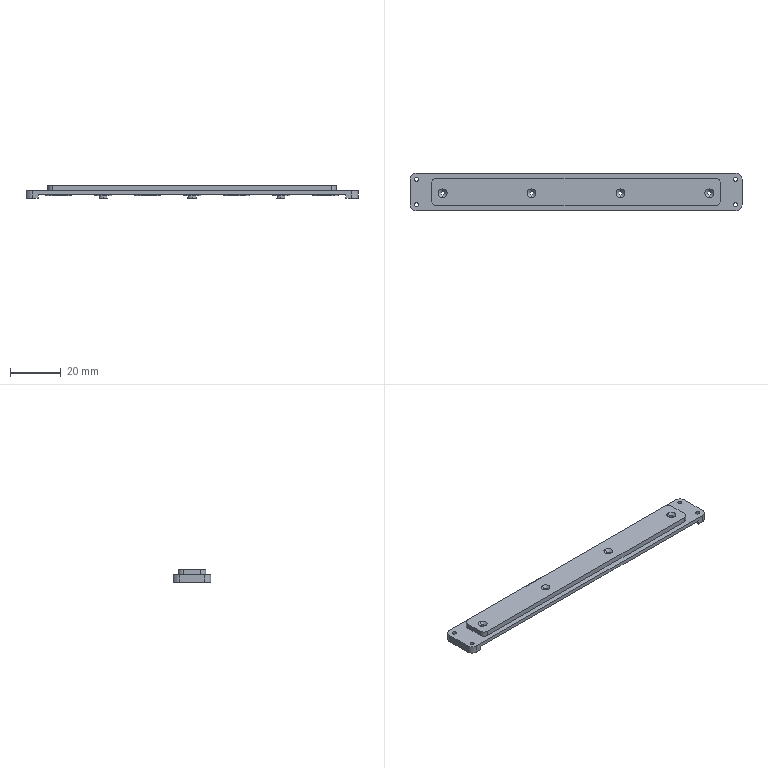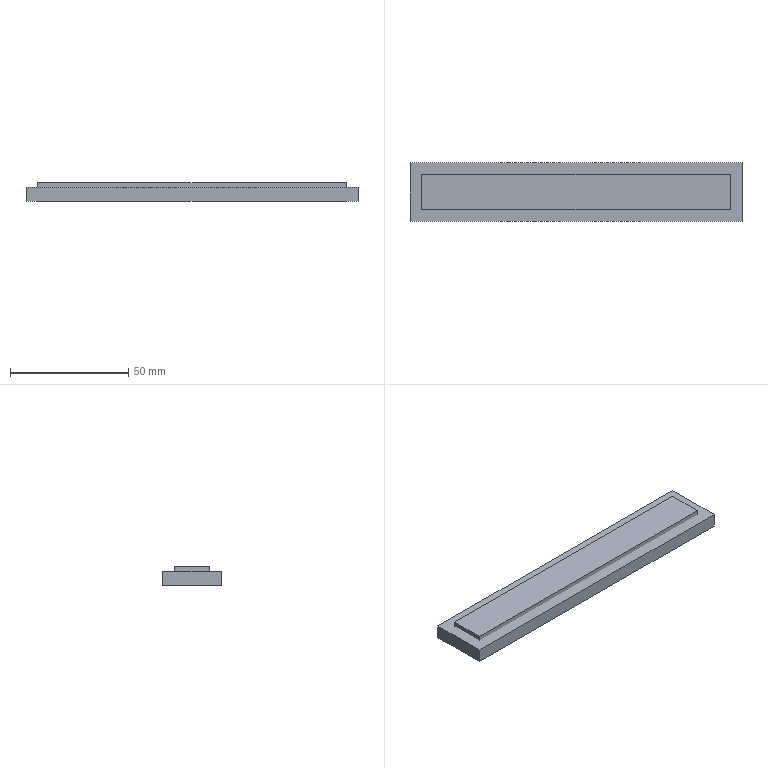CAM job | NX | 3-axis milling, drilling | part box 130.666 x 14.95 x 5 mm | stock box 140.666 x 24.95 x 8 mm
Tools:
number,name,description,diameter,corner_radius,flute_length,length,flutes
19,D80,Milling Tool-5 Parameters,80.0,0.0,50.0,75.0,2
1,D6A45,Milling Tool-5 Parameters,6.0,0.0,50.0,75.0,2
16,1.5ZT,Drilling Tool,1.5,0.0,35.0,50.0,2
17,1.6ZT,Drilling Tool,1.6,0.0,35.0,50.0,2
15,D10,Milling Tool-5 Parameters,10.0,0.0,50.0,75.0,2
14,D10JING,Milling Tool-5 Parameters,10.0,0.0,50.0,75.0,2
11,D4,Milling Tool-5 Parameters,4.0,0.0,50.0,75.0,2
2,D2,Milling Tool-5 Parameters,2.0,0.0,50.0,75.0,2
Operations:
program,operation,operation_type,tool,method,geometry_group,spindle_rpm,surface_speed,feed_per_tooth,feed_cut,feed_plunge,cut_length_mm,path_length_mm,cut_time_min,machine_time_min
1,FLOOR_WALL_COPY,VolumeBased25DMillingOperation,D80,METHOD,A,6500.0,1633.0,0.1154,1500.0,100.0,236.666,290.666,0.1578,0.1632
1,DRILLING_COPY_1,Operation,D6A45,METHOD,A,5000.0,94.0,0.035,350.0,0.0,38.0,306.457,0.1086,0.1354
1,DRILLING_COPY_1_COPY,Operation,1.5ZT,METHOD,A,2000.0,9.0,0.025,100.0,0.0,29.003,232.39,0.29,0.3104
1,DRILLING_COPY_1_COPY_COPY,Operation,1.6ZT,METHOD,A,2000.0,9.0,0.025,100.0,0.0,39.923,295.726,0.3992,0.4248
1,ADAPTIVE_MILLING,CavityMilling,D10,METHOD,A,9500.0,298.0,0.1579,3000.0,1000.0,3539.432,3666.063,1.184,1.196
1,ZLEVEL_PROFILE_COPY_1_COPY_COPY_1,ZLevelMilling,D10JING,METHOD,A,9500.0,298.0,0.0632,1200.0,1000.0,325.748,393.748,0.2721,0.2789
1,ZLEVEL_PROFILE_COPY_1_COPY_COPY_1_COPY,ZLevelMilling,D10JING,METHOD,A,9500.0,298.0,0.0632,1200.0,1000.0,284.366,346.366,0.2376,0.2438
1,PLANAR_MILL_COPY_COPY_COPY_COPY_COPY_COPY_1,PlanarMilling,D6A45,METHOD,A,9500.0,179.0,0.0658,1250.0,100.0,257.932,316.932,0.2063,0.2122
1,PLANAR_MILL_COPY_COPY_COPY_COPY_COPY_COPY_1_COPY,PlanarMilling,D6A45,METHOD,A,9500.0,179.0,0.0658,1250.0,100.0,308.731,374.731,0.247,0.2536
1,DRILLING_COPY_1_COPY_1,Operation,D6A45,METHOD,A,5000.0,94.0,0.035,350.0,0.0,16.4,252.287,0.0469,0.0704
2,FLOOR_WALL_COPY_COPY,VolumeBased25DMillingOperation,D80,METHOD,B,6500.0,1633.0,0.1154,1500.0,100.0,1359.997,2772.33,0.9067,1.048
2,DRILLING_COPY_1_COPY_2,Operation,D6A45,METHOD,B,5000.0,94.0,0.035,350.0,0.0,12.3,160.857,0.0351,0.05
2,DRILLING_COPY_1_COPY_COPY_COPY,Operation,1.6ZT,METHOD,B,2000.0,9.0,0.025,100.0,0.0,19.5,210.193,0.195,0.2141
2,CAVITY_MILL,CavityMilling,D10,METHOD,B,9500.0,298.0,0.1316,2500.0,1000.0,1194.511,1354.005,0.4908,0.5068
2,CAVITY_MILL_COPY,CavityMilling,D4,METHOD,B,9500.0,119.0,0.0789,1500.0,1000.0,1680.84,3159.425,1.443,1.591
2,FLOOR_WALL_COPY_1_COPY,VolumeBased25DMillingOperation,D4,METHOD,B,9500.0,298.0,0.0632,1200.0,1000.0,2207.783,3948.226,1.851,2.025
2,CAVITY_MILL_COPY_COPY,CavityMilling,D2,METHOD,B,9500.0,59.0,0.0579,1100.0,1000.0,1439.419,3093.97,1.344,1.509
2,PLANAR_MILL_COPY_COPY_COPY_COPY_COPY_COPY_1_COPY_1,PlanarMilling,D6A45,METHOD,B,9500.0,179.0,0.0658,1250.0,100.0,99.4,334.2,0.0795,0.103
2,PLANAR_MILL_COPY_COPY_COPY_COPY_COPY_COPY_1_COPY_1_COPY,PlanarMilling,D6A45,METHOD,B,9500.0,179.0,0.0658,1250.0,100.0,108.557,457.833,0.0868,0.1218
2,PLANAR_MILL_COPY_COPY_COPY_COPY_COPY_COPY_1_COPY_1_COPY_COPY,PlanarMilling,D6A45,METHOD,B,9500.0,179.0,0.0658,1250.0,100.0,243.202,386.811,0.1946,0.2089
2,DRILLING_COPY_1_COPY_1_COPY,Operation,D6A45,METHOD,B,5000.0,94.0,0.035,350.0,0.0,16.4,248.287,0.0469,0.07
2,DRILLING_COPY_1_COPY_1_COPY_COPY,Operation,D6A45,METHOD,B,5000.0,94.0,0.035,350.0,0.0,12.3,160.857,0.0351,0.05